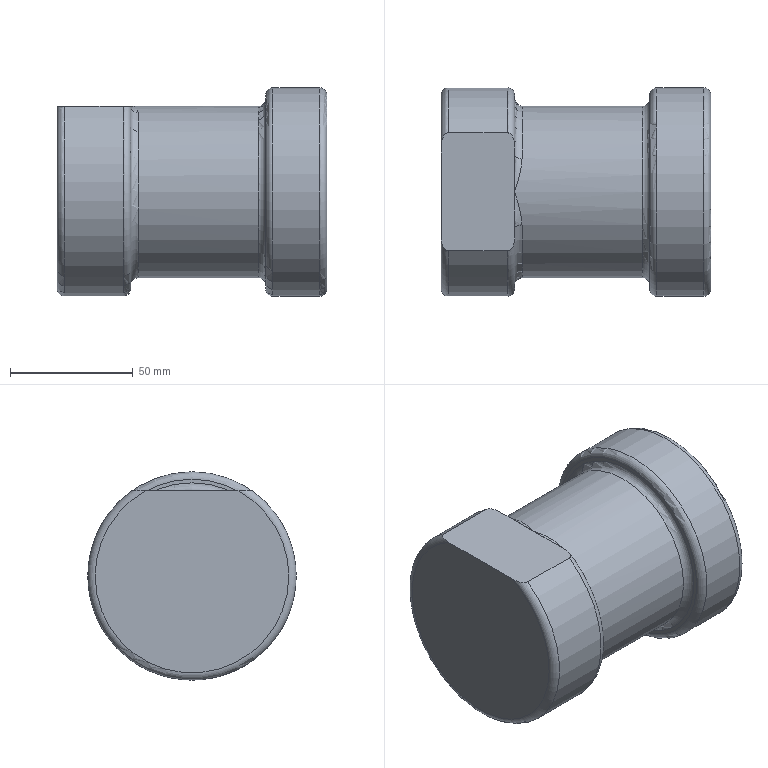Part | NX | features MAIN_BODY 2 | 1 solid | 19 faces | box 110 x 85 x 85 mm | volume 427132 mm3 | torus 6 | plane 5 | cylinder 4 | cone 2 | spline 2 | commonest cylinder face diameters 85 x2 34 x1 70 x1
STEP:
#1=CARTESIAN_POINT('',(1624.091,263.018,290.));
#2=VERTEX_POINT('',#1);
#3=CARTESIAN_POINT('',(1648.091,263.018,290.));
#4=VERTEX_POINT('',#3);
#5=CARTESIAN_POINT('',(1621.091,263.018,290.));
#6=DIRECTION('',(1.,0.,0.));
#7=VECTOR('',#6,1000.);
#8=LINE('',#5,#7);
#9=EDGE_CURVE('',#2,#4,#8,.T.);
#10=ORIENTED_EDGE('',*,*,#9,.T.);
#11=CARTESIAN_POINT('',(1648.091,214.8,290.));
#12=VERTEX_POINT('',#11);
#13=CARTESIAN_POINT('',(1648.091,238.909,255.));
#14=DIRECTION('',(1.,0.,0.));
#15=DIRECTION('',(0.,0.,1.));
#16=AXIS2_PLACEMENT_3D('',#13,#14,#15);
#17=CIRCLE('',#16,42.5);
#18=EDGE_CURVE('',#4,#12,#17,.F.);
#19=ORIENTED_EDGE('',*,*,#18,.T.);
#20=CARTESIAN_POINT('',(1624.091,214.8,290.));
#21=VERTEX_POINT('',#20);
#22=CARTESIAN_POINT('',(1621.091,214.8,290.));
#23=DIRECTION('',(1.,0.,0.));
#24=VECTOR('',#23,1000.);
#25=LINE('',#22,#24);
#26=EDGE_CURVE('',#12,#21,#25,.F.);
#27=ORIENTED_EDGE('',*,*,#26,.T.);
#28=CARTESIAN_POINT('',(1624.091,238.909,255.));
#29=DIRECTION('',(1.,0.,0.));
#30=DIRECTION('',(0.,0.,1.));
#31=AXIS2_PLACEMENT_3D('',#28,#29,#30);
#32=CIRCLE('',#31,42.5);
#33=EDGE_CURVE('',#21,#2,#32,.T.);
#34=ORIENTED_EDGE('',*,*,#33,.T.);
#35=EDGE_LOOP('',(#10,#19,#27,#34));
#36=FACE_BOUND('',#35,.T.);
#37=CARTESIAN_POINT('',(1731.091,238.909,255.));
#38=DIRECTION('',(-1.,0.,0.));
#39=DIRECTION('',(0.,0.,-1.));
#40=AXIS2_PLACEMENT_3D('',#37,#38,#39);
#41=CYLINDRICAL_SURFACE('',#40,42.5);
#42=ADVANCED_FACE('',(#36),#41,.T.);
#43=CARTESIAN_POINT('',(1621.091,257.219,290.));
#44=VERTEX_POINT('',#43);
#45=CARTESIAN_POINT('',(1621.091,220.599,290.));
#46=VERTEX_POINT('',#45);
#47=CARTESIAN_POINT('',(1621.091,263.018,290.));
#48=DIRECTION('',(0.,-1.,0.));
#49=VECTOR('',#48,1000.);
#50=LINE('',#47,#49);
#51=EDGE_CURVE('',#44,#46,#50,.T.);
#52=ORIENTED_EDGE('',*,*,#51,.F.);
#53=CARTESIAN_POINT('',(1621.091,238.909,255.));
#54=DIRECTION('',(1.,0.,0.));
#55=DIRECTION('',(0.,0.,1.));
#56=AXIS2_PLACEMENT_3D('',#53,#54,#55);
#57=CIRCLE('',#56,39.5);
#58=EDGE_CURVE('',#44,#46,#57,.F.);
#59=ORIENTED_EDGE('',*,*,#58,.T.);
#60=EDGE_LOOP('',(#52,#59));
#61=FACE_BOUND('',#60,.T.);
#62=CARTESIAN_POINT('',(1621.091,238.909,255.));
#63=DIRECTION('',(1.,0.,0.));
#64=DIRECTION('',(0.,0.,1.));
#65=AXIS2_PLACEMENT_3D('',#62,#63,#64);
#66=PLANE('',#65);
#67=ADVANCED_FACE('',(#61),#66,.F.);
#68=CARTESIAN_POINT('',(1651.091,257.219,290.));
#69=VERTEX_POINT('',#68);
#70=CARTESIAN_POINT('',(1651.091,253.708,290.));
#71=VERTEX_POINT('',#70);
#72=CARTESIAN_POINT('',(1651.091,238.909,290.));
#73=DIRECTION('',(0.,-1.,0.));
#74=VECTOR('',#73,1000.);
#75=LINE('',#72,#74);
#76=EDGE_CURVE('',#69,#71,#75,.T.);
#77=ORIENTED_EDGE('',*,*,#76,.T.);
#78=CARTESIAN_POINT('',(1651.091,224.11,290.));
#79=VERTEX_POINT('',#78);
#80=CARTESIAN_POINT('',(1651.091,238.909,255.));
#81=DIRECTION('',(1.,0.,0.));
#82=DIRECTION('',(0.,0.,1.));
#83=AXIS2_PLACEMENT_3D('',#80,#81,#82);
#84=CIRCLE('',#83,38.);
#85=EDGE_CURVE('',#71,#79,#84,.F.);
#86=ORIENTED_EDGE('',*,*,#85,.T.);
#87=CARTESIAN_POINT('',(1651.091,220.599,290.));
#88=VERTEX_POINT('',#87);
#89=CARTESIAN_POINT('',(1651.091,238.909,290.));
#90=DIRECTION('',(0.,-1.,0.));
#91=VECTOR('',#90,1000.);
#92=LINE('',#89,#91);
#93=EDGE_CURVE('',#79,#88,#92,.T.);
#94=ORIENTED_EDGE('',*,*,#93,.T.);
#95=CARTESIAN_POINT('',(1651.091,238.909,255.));
#96=DIRECTION('',(1.,0.,0.));
#97=DIRECTION('',(0.,0.,1.));
#98=AXIS2_PLACEMENT_3D('',#95,#96,#97);
#99=CIRCLE('',#98,39.5);
#100=EDGE_CURVE('',#88,#69,#99,.T.);
#101=ORIENTED_EDGE('',*,*,#100,.T.);
#102=EDGE_LOOP('',(#77,#86,#94,#101));
#103=FACE_BOUND('',#102,.T.);
#104=CARTESIAN_POINT('',(1651.091,238.909,255.));
#105=DIRECTION('',(1.,0.,0.));
#106=DIRECTION('',(0.,0.,1.));
#107=AXIS2_PLACEMENT_3D('',#104,#105,#106);
#108=PLANE('',#107);
#109=ADVANCED_FACE('',(#103),#108,.T.);
#110=ORIENTED_EDGE('',*,*,#58,.F.);
#111=CARTESIAN_POINT('',(1621.091,257.219,290.));
#112=CARTESIAN_POINT('',(1621.091,258.399,290.));
#113=CARTESIAN_POINT('',(1621.296,260.185,290.));
#114=CARTESIAN_POINT('',(1622.401,262.344,290.));
#115=CARTESIAN_POINT('',(1623.489,263.018,290.));
#116=CARTESIAN_POINT('',(1624.091,263.018,290.));
#117=B_SPLINE_CURVE_WITH_KNOTS('',3,(#111,#112,#113,#114,#115,#116),.UNSPECIFIED.,.F.,.F.,(4,1,1,4),(0.02726,0.03083,0.03261,0.0344),.UNSPECIFIED.);
#118=EDGE_CURVE('',#44,#2,#117,.T.);
#119=ORIENTED_EDGE('',*,*,#118,.T.);
#120=ORIENTED_EDGE('',*,*,#33,.F.);
#121=CARTESIAN_POINT('',(1624.091,214.8,290.));
#122=CARTESIAN_POINT('',(1623.497,214.8,290.));
#123=CARTESIAN_POINT('',(1622.393,215.48,290.));
#124=CARTESIAN_POINT('',(1621.573,217.093,290.));
#125=CARTESIAN_POINT('',(1621.163,218.828,290.));
#126=CARTESIAN_POINT('',(1621.091,220.011,290.));
#127=CARTESIAN_POINT('',(1621.091,220.599,290.));
#128=B_SPLINE_CURVE_WITH_KNOTS('',3,(#121,#122,#123,#124,#125,#126,#127),.UNSPECIFIED.,.F.,.F.,(4,1,1,1,4),(0.01599,0.01778,0.01957,0.02137,0.02316),.UNSPECIFIED.);
#129=EDGE_CURVE('',#21,#46,#128,.T.);
#130=ORIENTED_EDGE('',*,*,#129,.T.);
#131=EDGE_LOOP('',(#110,#119,#120,#130));
#132=FACE_BOUND('',#131,.T.);
#133=CARTESIAN_POINT('',(1624.091,238.909,255.));
#134=DIRECTION('',(1.,0.,0.));
#135=DIRECTION('',(0.,0.,1.));
#136=AXIS2_PLACEMENT_3D('',#133,#134,#135);
#137=TOROIDAL_SURFACE('',#136,39.5,3.);
#138=ADVANCED_FACE('',(#132),#137,.T.);
#139=CARTESIAN_POINT('',(1706.091,238.909,293.));
#140=VERTEX_POINT('',#139);
#141=CARTESIAN_POINT('',(1706.091,238.909,255.));
#142=DIRECTION('',(1.,0.,0.));
#143=DIRECTION('',(0.,0.,1.));
#144=AXIS2_PLACEMENT_3D('',#141,#142,#143);
#145=CIRCLE('',#144,38.);
#146=EDGE_CURVE('',#140,#140,#145,.T.);
#147=ORIENTED_EDGE('',*,*,#146,.T.);
#148=EDGE_LOOP('',(#147));
#149=FACE_BOUND('',#148,.T.);
#150=CARTESIAN_POINT('',(1706.091,238.909,294.5));
#151=VERTEX_POINT('',#150);
#152=CARTESIAN_POINT('',(1706.091,238.909,255.));
#153=DIRECTION('',(1.,0.,0.));
#154=DIRECTION('',(0.,0.,1.));
#155=AXIS2_PLACEMENT_3D('',#152,#153,#154);
#156=CIRCLE('',#155,39.5);
#157=EDGE_CURVE('',#151,#151,#156,.F.);
#158=ORIENTED_EDGE('',*,*,#157,.T.);
#159=EDGE_LOOP('',(#158));
#160=FACE_BOUND('',#159,.T.);
#161=CARTESIAN_POINT('',(1706.091,238.909,255.));
#162=DIRECTION('',(1.,0.,0.));
#163=DIRECTION('',(0.,0.,1.));
#164=AXIS2_PLACEMENT_3D('',#161,#162,#163);
#165=PLANE('',#164);
#166=ADVANCED_FACE('',(#149,#160),#165,.F.);
#167=CARTESIAN_POINT('',(1703.091,238.909,290.));
#168=VERTEX_POINT('',#167);
#169=CARTESIAN_POINT('',(1703.091,238.909,255.));
#170=DIRECTION('',(1.,0.,0.));
#171=DIRECTION('',(0.,0.,1.));
#172=AXIS2_PLACEMENT_3D('',#169,#170,#171);
#173=CIRCLE('',#172,35.);
#174=EDGE_CURVE('',#168,#168,#173,.F.);
#175=ORIENTED_EDGE('',*,*,#174,.T.);
#176=EDGE_LOOP('',(#175));
#177=FACE_BOUND('',#176,.T.);
#178=CARTESIAN_POINT('',(1654.091,252.539,287.237));
#179=VERTEX_POINT('',#178);
#180=CARTESIAN_POINT('',(1651.091,238.909,290.));
#181=VERTEX_POINT('',#180);
#182=CARTESIAN_POINT('',(1654.091,252.539,287.237));
#183=CARTESIAN_POINT('',(1654.091,250.317,288.176));
#184=CARTESIAN_POINT('',(1653.18,245.775,289.555));
#185=CARTESIAN_POINT('',(1651.789,241.196,290.));
#186=CARTESIAN_POINT('',(1651.091,238.909,290.));
#187=B_SPLINE_CURVE_WITH_KNOTS('',3,(#182,#183,#184,#185,#186),.UNSPECIFIED.,.F.,.F.,(4,1,4),(0.,0.007173,0.01435),.UNSPECIFIED.);
#188=EDGE_CURVE('',#179,#181,#187,.T.);
#189=ORIENTED_EDGE('',*,*,#188,.T.);
#190=CARTESIAN_POINT('',(1654.091,225.279,287.237));
#191=VERTEX_POINT('',#190);
#192=CARTESIAN_POINT('',(1654.091,225.279,287.237));
#193=CARTESIAN_POINT('',(1654.091,227.501,288.176));
#194=CARTESIAN_POINT('',(1653.18,232.043,289.555));
#195=CARTESIAN_POINT('',(1651.789,236.622,290.));
#196=CARTESIAN_POINT('',(1651.091,238.909,290.));
#197=B_SPLINE_CURVE_WITH_KNOTS('',3,(#192,#193,#194,#195,#196),.UNSPECIFIED.,.F.,.F.,(4,1,4),(0.,0.007173,0.01435),.UNSPECIFIED.);
#198=EDGE_CURVE('',#181,#191,#197,.F.);
#199=ORIENTED_EDGE('',*,*,#198,.T.);
#200=CARTESIAN_POINT('',(1654.091,238.909,255.));
#201=DIRECTION('',(1.,0.,0.));
#202=DIRECTION('',(0.,0.,1.));
#203=AXIS2_PLACEMENT_3D('',#200,#201,#202);
#204=CIRCLE('',#203,35.);
#205=EDGE_CURVE('',#191,#179,#204,.T.);
#206=ORIENTED_EDGE('',*,*,#205,.T.);
#207=EDGE_LOOP('',(#189,#199,#206));
#208=FACE_BOUND('',#207,.T.);
#209=CARTESIAN_POINT('',(1678.591,238.909,255.));
#210=DIRECTION('',(1.,0.,0.));
#211=DIRECTION('',(0.,0.,1.));
#212=AXIS2_PLACEMENT_3D('',#209,#210,#211);
#213=CYLINDRICAL_SURFACE('',#212,35.);
#214=ADVANCED_FACE('',(#177,#208),#213,.T.);
#215=CARTESIAN_POINT('',(1731.091,238.909,294.5));
#216=VERTEX_POINT('',#215);
#217=CARTESIAN_POINT('',(1731.091,238.909,255.));
#218=DIRECTION('',(1.,0.,0.));
#219=DIRECTION('',(0.,0.,1.));
#220=AXIS2_PLACEMENT_3D('',#217,#218,#219);
#221=CIRCLE('',#220,39.5);
#222=EDGE_CURVE('',#216,#216,#221,.T.);
#223=ORIENTED_EDGE('',*,*,#222,.T.);
#224=EDGE_LOOP('',(#223));
#225=FACE_BOUND('',#224,.T.);
#226=CARTESIAN_POINT('',(1731.091,238.909,231.));
#227=VERTEX_POINT('',#226);
#228=CARTESIAN_POINT('',(1731.091,238.909,255.));
#229=DIRECTION('',(-1.,0.,0.));
#230=DIRECTION('',(0.,0.,-1.));
#231=AXIS2_PLACEMENT_3D('',#228,#229,#230);
#232=CIRCLE('',#231,24.);
#233=EDGE_CURVE('',#227,#227,#232,.T.);
#234=ORIENTED_EDGE('',*,*,#233,.T.);
#235=EDGE_LOOP('',(#234));
#236=FACE_BOUND('',#235,.T.);
#237=CARTESIAN_POINT('',(1731.091,238.909,255.));
#238=DIRECTION('',(1.,0.,0.));
#239=DIRECTION('',(0.,0.,1.));
#240=AXIS2_PLACEMENT_3D('',#237,#238,#239);
#241=PLANE('',#240);
#242=ADVANCED_FACE('',(#225,#236),#241,.T.);
#243=CARTESIAN_POINT('',(1728.091,238.909,297.5));
#244=VERTEX_POINT('',#243);
#245=CARTESIAN_POINT('',(1728.091,238.909,255.));
#246=DIRECTION('',(1.,0.,0.));
#247=DIRECTION('',(0.,0.,1.));
#248=AXIS2_PLACEMENT_3D('',#245,#246,#247);
#249=CIRCLE('',#248,42.5);
#250=EDGE_CURVE('',#244,#244,#249,.F.);
#251=ORIENTED_EDGE('',*,*,#250,.T.);
#252=EDGE_LOOP('',(#251));
#253=FACE_BOUND('',#252,.T.);
#254=CARTESIAN_POINT('',(1709.091,238.909,297.5));
#255=VERTEX_POINT('',#254);
#256=CARTESIAN_POINT('',(1709.091,238.909,255.));
#257=DIRECTION('',(1.,0.,0.));
#258=DIRECTION('',(0.,0.,1.));
#259=AXIS2_PLACEMENT_3D('',#256,#257,#258);
#260=CIRCLE('',#259,42.5);
#261=EDGE_CURVE('',#255,#255,#260,.T.);
#262=ORIENTED_EDGE('',*,*,#261,.T.);
#263=EDGE_LOOP('',(#262));
#264=FACE_BOUND('',#263,.T.);
#265=CARTESIAN_POINT('',(1731.091,238.909,255.));
#266=DIRECTION('',(-1.,0.,0.));
#267=DIRECTION('',(0.,0.,-1.));
#268=AXIS2_PLACEMENT_3D('',#265,#266,#267);
#269=CYLINDRICAL_SURFACE('',#268,42.5);
#270=ADVANCED_FACE('',(#253,#264),#269,.T.);
#271=CARTESIAN_POINT('',(1641.091,238.909,238.));
#272=VERTEX_POINT('',#271);
#273=CARTESIAN_POINT('',(1641.091,238.909,255.));
#274=DIRECTION('',(-1.,0.,0.));
#275=DIRECTION('',(0.,0.,-1.));
#276=AXIS2_PLACEMENT_3D('',#273,#274,#275);
#277=CIRCLE('',#276,17.);
#278=EDGE_CURVE('',#272,#272,#277,.T.);
#279=ORIENTED_EDGE('',*,*,#278,.F.);
#280=EDGE_LOOP('',(#279));
#281=FACE_BOUND('',#280,.T.);
#282=CARTESIAN_POINT('',(1636.536,238.909,255.));
#283=VERTEX_POINT('',#282);
#284=VERTEX_LOOP('',#283);
#285=FACE_BOUND('',#284,.T.);
#286=CARTESIAN_POINT('',(1641.091,238.909,255.));
#287=DIRECTION('',(1.,0.,0.));
#288=DIRECTION('',(0.,0.,1.));
#289=AXIS2_PLACEMENT_3D('',#286,#287,#288);
#290=CONICAL_SURFACE('',#289,17.,1.309);
#291=ADVANCED_FACE('',(#281,#285),#290,.F.);
#292=ORIENTED_EDGE('',*,*,#278,.T.);
#293=EDGE_LOOP('',(#292));
#294=FACE_BOUND('',#293,.T.);
#295=CARTESIAN_POINT('',(1718.967,238.909,238.));
#296=VERTEX_POINT('',#295);
#297=CARTESIAN_POINT('',(1718.967,238.909,255.));
#298=DIRECTION('',(-1.,0.,0.));
#299=DIRECTION('',(0.,0.,-1.));
#300=AXIS2_PLACEMENT_3D('',#297,#298,#299);
#301=CIRCLE('',#300,17.);
#302=EDGE_CURVE('',#296,#296,#301,.T.);
#303=ORIENTED_EDGE('',*,*,#302,.F.);
#304=EDGE_LOOP('',(#303));
#305=FACE_BOUND('',#304,.T.);
#306=CARTESIAN_POINT('',(1641.091,238.909,255.));
#307=DIRECTION('',(-1.,0.,0.));
#308=DIRECTION('',(0.,0.,-1.));
#309=AXIS2_PLACEMENT_3D('',#306,#307,#308);
#310=CYLINDRICAL_SURFACE('',#309,17.);
#311=ADVANCED_FACE('',(#294,#305),#310,.F.);
#312=ORIENTED_EDGE('',*,*,#302,.T.);
#313=EDGE_LOOP('',(#312));
#314=FACE_BOUND('',#313,.T.);
#315=ORIENTED_EDGE('',*,*,#233,.F.);
#316=EDGE_LOOP('',(#315));
#317=FACE_BOUND('',#316,.T.);
#318=CARTESIAN_POINT('',(1731.091,238.909,255.));
#319=DIRECTION('',(1.,0.,0.));
#320=DIRECTION('',(0.,0.,1.));
#321=AXIS2_PLACEMENT_3D('',#318,#319,#320);
#322=CONICAL_SURFACE('',#321,24.,0.5236);
#323=ADVANCED_FACE('',(#314,#317),#322,.F.);
#324=ORIENTED_EDGE('',*,*,#76,.F.);
#325=CARTESIAN_POINT('',(1651.091,257.219,290.));
#326=CARTESIAN_POINT('',(1651.091,258.408,290.));
#327=CARTESIAN_POINT('',(1650.882,260.19,290.));
#328=CARTESIAN_POINT('',(1649.782,262.342,290.));
#329=CARTESIAN_POINT('',(1648.693,263.018,290.));
#330=CARTESIAN_POINT('',(1648.091,263.018,290.));
#331=B_SPLINE_CURVE_WITH_KNOTS('',3,(#325,#326,#327,#328,#329,#330),.UNSPECIFIED.,.F.,.F.,(4,1,1,4),(0.,0.003537,0.005305,0.007074),.UNSPECIFIED.);
#332=EDGE_CURVE('',#69,#4,#331,.T.);
#333=ORIENTED_EDGE('',*,*,#332,.T.);
#334=ORIENTED_EDGE('',*,*,#9,.F.);
#335=ORIENTED_EDGE('',*,*,#118,.F.);
#336=ORIENTED_EDGE('',*,*,#51,.T.);
#337=ORIENTED_EDGE('',*,*,#129,.F.);
#338=ORIENTED_EDGE('',*,*,#26,.F.);
#339=CARTESIAN_POINT('',(1648.091,214.8,290.));
#340=CARTESIAN_POINT('',(1648.695,214.8,290.));
#341=CARTESIAN_POINT('',(1649.781,215.476,290.));
#342=CARTESIAN_POINT('',(1650.881,217.623,290.));
#343=CARTESIAN_POINT('',(1651.091,219.41,290.));
#344=CARTESIAN_POINT('',(1651.091,220.599,290.));
#345=B_SPLINE_CURVE_WITH_KNOTS('',3,(#339,#340,#341,#342,#343,#344),.UNSPECIFIED.,.F.,.F.,(4,1,1,4),(0.,0.001776,0.003553,0.007105),.UNSPECIFIED.);
#346=EDGE_CURVE('',#12,#88,#345,.T.);
#347=ORIENTED_EDGE('',*,*,#346,.T.);
#348=ORIENTED_EDGE('',*,*,#93,.F.);
#349=CARTESIAN_POINT('',(1651.091,238.909,290.));
#350=DIRECTION('',(0.,-1.,0.));
#351=VECTOR('',#350,1000.);
#352=LINE('',#349,#351);
#353=EDGE_CURVE('',#181,#79,#352,.T.);
#354=ORIENTED_EDGE('',*,*,#353,.F.);
#355=CARTESIAN_POINT('',(1651.091,238.909,290.));
#356=DIRECTION('',(0.,-1.,0.));
#357=VECTOR('',#356,1000.);
#358=LINE('',#355,#357);
#359=EDGE_CURVE('',#71,#181,#358,.T.);
#360=ORIENTED_EDGE('',*,*,#359,.F.);
#361=EDGE_LOOP('',(#324,#333,#334,#335,#336,#337,#338,#347,#348,#354,#360));
#362=FACE_BOUND('',#361,.T.);
#363=CARTESIAN_POINT('',(1621.091,263.018,290.));
#364=DIRECTION('',(0.,0.,1.));
#365=DIRECTION('',(-1.,0.,0.));
#366=AXIS2_PLACEMENT_3D('',#363,#364,#365);
#367=PLANE('',#366);
#368=ADVANCED_FACE('',(#362),#367,.T.);
#369=ORIENTED_EDGE('',*,*,#250,.F.);
#370=EDGE_LOOP('',(#369));
#371=FACE_BOUND('',#370,.T.);
#372=ORIENTED_EDGE('',*,*,#222,.F.);
#373=EDGE_LOOP('',(#372));
#374=FACE_BOUND('',#373,.T.);
#375=CARTESIAN_POINT('',(1728.091,238.909,255.));
#376=DIRECTION('',(1.,0.,0.));
#377=DIRECTION('',(0.,0.,1.));
#378=AXIS2_PLACEMENT_3D('',#375,#376,#377);
#379=TOROIDAL_SURFACE('',#378,39.5,3.);
#380=ADVANCED_FACE('',(#371,#374),#379,.T.);
#381=ORIENTED_EDGE('',*,*,#359,.T.);
#382=ORIENTED_EDGE('',*,*,#188,.F.);
#383=CARTESIAN_POINT('',(1654.091,253.708,290.));
#384=DIRECTION('',(0.,0.9211,-0.3894));
#385=DIRECTION('',(0.,0.3894,0.9211));
#386=AXIS2_PLACEMENT_3D('',#383,#384,#385);
#387=CIRCLE('',#386,3.);
#388=EDGE_CURVE('',#71,#179,#387,.F.);
#389=ORIENTED_EDGE('',*,*,#388,.F.);
#390=EDGE_LOOP('',(#381,#382,#389));
#391=FACE_BOUND('',#390,.T.);
#392=CARTESIAN_POINT('',(1654.091,252.539,287.237));
#393=CARTESIAN_POINT('',(1651.091,252.539,287.237));
#394=CARTESIAN_POINT('',(1651.091,253.708,290.));
#395=CARTESIAN_POINT('',(1654.091,251.437,287.703));
#396=CARTESIAN_POINT('',(1651.524,251.685,287.598));
#397=CARTESIAN_POINT('',(1651.091,252.511,290.));
#398=CARTESIAN_POINT('',(1653.849,249.21,288.513));
#399=CARTESIAN_POINT('',(1651.997,249.65,288.376));
#400=CARTESIAN_POINT('',(1651.091,250.093,290.));
#401=CARTESIAN_POINT('',(1652.843,244.626,289.667));
#402=CARTESIAN_POINT('',(1651.993,245.088,289.589));
#403=CARTESIAN_POINT('',(1651.091,245.116,290.));
#404=CARTESIAN_POINT('',(1651.801,241.236,290.));
#405=CARTESIAN_POINT('',(1651.446,241.336,290.));
#406=CARTESIAN_POINT('',(1651.091,241.436,290.));
#407=CARTESIAN_POINT('',(1651.091,238.909,290.));
#408=CARTESIAN_POINT('',(1651.091,238.909,290.));
#409=CARTESIAN_POINT('',(1651.091,238.909,290.));
#410=(BOUNDED_SURFACE()B_SPLINE_SURFACE(3,2,((#392,#393,#394),(#395,#396,#397),(#398,#399,#400),(#401,#402,#403),(#404,#405,#406),(#407,#408,#409)),.UNSPECIFIED.,.F.,.F.,.F.)B_SPLINE_SURFACE_WITH_KNOTS((4,1,1,4),(3,3),(0.007753,0.01169,0.01563,0.0235),(0.,1.),.UNSPECIFIED.)GEOMETRIC_REPRESENTATION_ITEM()RATIONAL_B_SPLINE_SURFACE(((1.,0.7071,1.),(1.,0.7621,1.),(1.,0.8504,1.),(1.,0.9683,1.),(1.,1.,1.),(1.,1.,1.)))REPRESENTATION_ITEM('')SURFACE());
#411=ADVANCED_FACE('',(#391),#410,.F.);
#412=ORIENTED_EDGE('',*,*,#388,.T.);
#413=ORIENTED_EDGE('',*,*,#205,.F.);
#414=CARTESIAN_POINT('',(1654.091,224.11,290.));
#415=DIRECTION('',(0.,-0.9211,-0.3894));
#416=DIRECTION('',(0.,0.3894,-0.9211));
#417=AXIS2_PLACEMENT_3D('',#414,#415,#416);
#418=CIRCLE('',#417,3.);
#419=EDGE_CURVE('',#79,#191,#418,.T.);
#420=ORIENTED_EDGE('',*,*,#419,.F.);
#421=ORIENTED_EDGE('',*,*,#85,.F.);
#422=EDGE_LOOP('',(#412,#413,#420,#421));
#423=FACE_BOUND('',#422,.T.);
#424=CARTESIAN_POINT('',(1654.091,238.909,255.));
#425=DIRECTION('',(1.,0.,0.));
#426=DIRECTION('',(0.,0.,1.));
#427=AXIS2_PLACEMENT_3D('',#424,#425,#426);
#428=TOROIDAL_SURFACE('',#427,38.,3.);
#429=ADVANCED_FACE('',(#423),#428,.F.);
#430=ORIENTED_EDGE('',*,*,#198,.F.);
#431=ORIENTED_EDGE('',*,*,#353,.T.);
#432=ORIENTED_EDGE('',*,*,#419,.T.);
#433=EDGE_LOOP('',(#430,#431,#432));
#434=FACE_BOUND('',#433,.T.);
#435=CARTESIAN_POINT('',(1651.091,224.11,290.));
#436=CARTESIAN_POINT('',(1651.091,225.279,287.237));
#437=CARTESIAN_POINT('',(1654.091,225.279,287.237));
#438=CARTESIAN_POINT('',(1651.091,225.308,290.));
#439=CARTESIAN_POINT('',(1651.524,226.133,287.598));
#440=CARTESIAN_POINT('',(1654.091,226.381,287.703));
#441=CARTESIAN_POINT('',(1651.091,227.726,290.));
#442=CARTESIAN_POINT('',(1651.997,228.168,288.376));
#443=CARTESIAN_POINT('',(1653.849,228.608,288.513));
#444=CARTESIAN_POINT('',(1651.091,232.702,290.));
#445=CARTESIAN_POINT('',(1651.993,232.73,289.589));
#446=CARTESIAN_POINT('',(1652.843,233.192,289.667));
#447=CARTESIAN_POINT('',(1651.091,236.383,290.));
#448=CARTESIAN_POINT('',(1651.446,236.482,290.));
#449=CARTESIAN_POINT('',(1651.801,236.582,290.));
#450=CARTESIAN_POINT('',(1651.091,238.909,290.));
#451=CARTESIAN_POINT('',(1651.091,238.909,290.));
#452=CARTESIAN_POINT('',(1651.091,238.909,290.));
#453=(BOUNDED_SURFACE()B_SPLINE_SURFACE(3,2,((#435,#436,#437),(#438,#439,#440),(#441,#442,#443),(#444,#445,#446),(#447,#448,#449),(#450,#451,#452)),.UNSPECIFIED.,.F.,.F.,.F.)B_SPLINE_SURFACE_WITH_KNOTS((4,1,1,4),(3,3),(0.007753,0.01169,0.01563,0.0235),(0.,1.),.UNSPECIFIED.)GEOMETRIC_REPRESENTATION_ITEM()RATIONAL_B_SPLINE_SURFACE(((1.,0.7071,1.),(1.,0.7621,1.),(1.,0.8504,1.),(1.,0.9683,1.),(1.,1.,1.),(1.,1.,1.)))REPRESENTATION_ITEM('')SURFACE());
#454=ADVANCED_FACE('',(#434),#453,.F.);
#455=ORIENTED_EDGE('',*,*,#346,.F.);
#456=ORIENTED_EDGE('',*,*,#18,.F.);
#457=ORIENTED_EDGE('',*,*,#332,.F.);
#458=ORIENTED_EDGE('',*,*,#100,.F.);
#459=EDGE_LOOP('',(#455,#456,#457,#458));
#460=FACE_BOUND('',#459,.T.);
#461=CARTESIAN_POINT('',(1648.091,238.909,255.));
#462=DIRECTION('',(1.,0.,0.));
#463=DIRECTION('',(0.,0.,1.));
#464=AXIS2_PLACEMENT_3D('',#461,#462,#463);
#465=TOROIDAL_SURFACE('',#464,39.5,3.);
#466=ADVANCED_FACE('',(#460),#465,.T.);
#467=ORIENTED_EDGE('',*,*,#174,.F.);
#468=EDGE_LOOP('',(#467));
#469=FACE_BOUND('',#468,.T.);
#470=ORIENTED_EDGE('',*,*,#146,.F.);
#471=EDGE_LOOP('',(#470));
#472=FACE_BOUND('',#471,.T.);
#473=CARTESIAN_POINT('',(1703.091,238.909,255.));
#474=DIRECTION('',(1.,0.,0.));
#475=DIRECTION('',(0.,0.,1.));
#476=AXIS2_PLACEMENT_3D('',#473,#474,#475);
#477=TOROIDAL_SURFACE('',#476,38.,3.);
#478=ADVANCED_FACE('',(#469,#472),#477,.F.);
#479=ORIENTED_EDGE('',*,*,#157,.F.);
#480=EDGE_LOOP('',(#479));
#481=FACE_BOUND('',#480,.T.);
#482=ORIENTED_EDGE('',*,*,#261,.F.);
#483=EDGE_LOOP('',(#482));
#484=FACE_BOUND('',#483,.T.);
#485=CARTESIAN_POINT('',(1709.091,238.909,255.));
#486=DIRECTION('',(1.,0.,0.));
#487=DIRECTION('',(0.,0.,1.));
#488=AXIS2_PLACEMENT_3D('',#485,#486,#487);
#489=TOROIDAL_SURFACE('',#488,39.5,3.);
#490=ADVANCED_FACE('',(#481,#484),#489,.T.);
#491=CLOSED_SHELL('',(#42,#67,#109,#138,#166,#214,#242,#270,#291,#311,#323,#368,#380,#411,#429,#454,#466,#478,#490));
#492=MANIFOLD_SOLID_BREP('',#491);
#493=(LENGTH_UNIT()NAMED_UNIT(*)SI_UNIT(.MILLI.,.METRE.));
#494=UNCERTAINTY_MEASURE_WITH_UNIT(LENGTH_MEASURE(0.0508),#493,'','');
#495=(NAMED_UNIT(*)PLANE_ANGLE_UNIT()SI_UNIT($,.RADIAN.));
#496=(NAMED_UNIT(*)SI_UNIT($,.STERADIAN.)SOLID_ANGLE_UNIT());
#497=(GEOMETRIC_REPRESENTATION_CONTEXT(3)GLOBAL_UNCERTAINTY_ASSIGNED_CONTEXT((#494))GLOBAL_UNIT_ASSIGNED_CONTEXT((#493,#495,#496))REPRESENTATION_CONTEXT('',''));
#498=ADVANCED_BREP_SHAPE_REPRESENTATION('',(#492),#497);